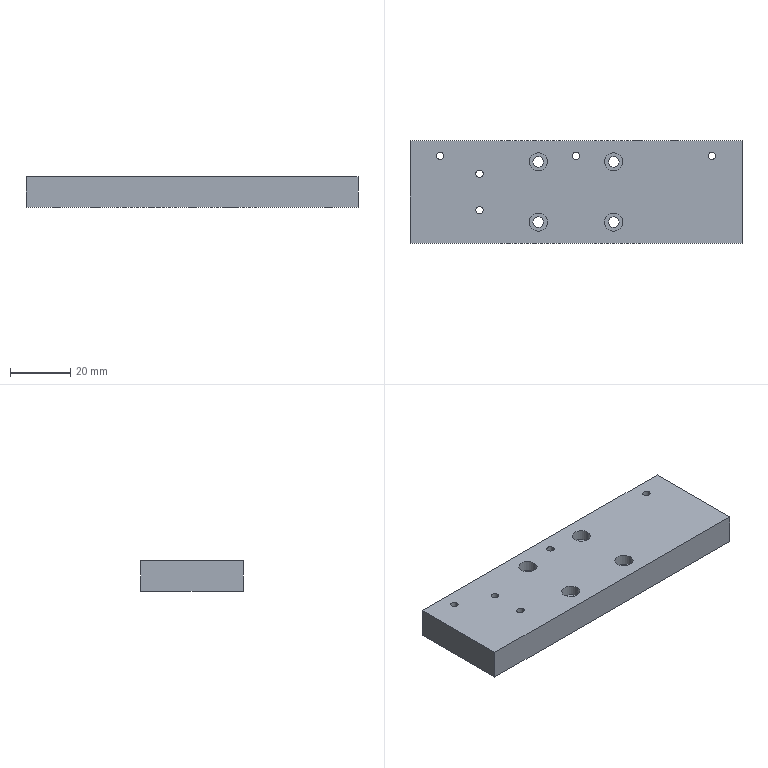Part | SolidWorks | features BaseBody 1 | 1 solid | 44 faces | box 110 x 34 x 10 mm | volume 36400 mm3 | cylinder 30 | plane 10 | cone 4 | commonest cylinder face diameters 2.459 x14 3.5 x8 6 x8
STEP:
#1=CARTESIAN_POINT('',(-17.191,-0.5864,0.));
#2=VERTEX_POINT('',#1);
#3=CARTESIAN_POINT('',(-20.691,-0.5864,0.));
#4=VERTEX_POINT('',#3);
#5=CARTESIAN_POINT('',(-18.941,-0.5864,0.));
#6=DIRECTION('',(0.,0.,-1.));
#7=DIRECTION('',(1.,0.,0.));
#8=AXIS2_PLACEMENT_3D('',#5,#6,#7);
#9=CIRCLE('',#8,1.75);
#10=EDGE_CURVE('',#2,#4,#9,.T.);
#11=ORIENTED_EDGE('',*,*,#10,.T.);
#12=CARTESIAN_POINT('',(-20.691,-0.5864,6.5));
#13=VERTEX_POINT('',#12);
#14=CARTESIAN_POINT('',(-20.691,-0.5864,-105.568));
#15=DIRECTION('',(0.,0.,1.));
#16=VECTOR('',#15,1000.);
#17=LINE('',#14,#16);
#18=EDGE_CURVE('',#4,#13,#17,.T.);
#19=ORIENTED_EDGE('',*,*,#18,.T.);
#20=CARTESIAN_POINT('',(-17.191,-0.5864,6.5));
#21=VERTEX_POINT('',#20);
#22=CARTESIAN_POINT('',(-18.941,-0.5864,6.5));
#23=DIRECTION('',(0.,0.,-1.));
#24=DIRECTION('',(1.,0.,0.));
#25=AXIS2_PLACEMENT_3D('',#22,#23,#24);
#26=CIRCLE('',#25,1.75);
#27=EDGE_CURVE('',#21,#13,#26,.T.);
#28=ORIENTED_EDGE('',*,*,#27,.F.);
#29=CARTESIAN_POINT('',(-17.191,-0.5864,-105.568));
#30=DIRECTION('',(0.,0.,1.));
#31=VECTOR('',#30,1000.);
#32=LINE('',#29,#31);
#33=EDGE_CURVE('',#2,#21,#32,.T.);
#34=ORIENTED_EDGE('',*,*,#33,.F.);
#35=EDGE_LOOP('',(#11,#19,#28,#34));
#36=FACE_OUTER_BOUND('',#35,.T.);
#37=CARTESIAN_POINT('',(-18.941,-0.5864,-105.568));
#38=DIRECTION('',(0.,0.,1.));
#39=DIRECTION('',(1.,0.,0.));
#40=AXIS2_PLACEMENT_3D('',#37,#38,#39);
#41=CYLINDRICAL_SURFACE('',#40,1.75);
#42=ADVANCED_FACE('',(#36),#41,.F.);
#43=CARTESIAN_POINT('',(7.809,-0.5864,0.));
#44=VERTEX_POINT('',#43);
#45=CARTESIAN_POINT('',(4.309,-0.5864,0.));
#46=VERTEX_POINT('',#45);
#47=CARTESIAN_POINT('',(6.059,-0.5864,0.));
#48=DIRECTION('',(0.,0.,-1.));
#49=DIRECTION('',(1.,0.,0.));
#50=AXIS2_PLACEMENT_3D('',#47,#48,#49);
#51=CIRCLE('',#50,1.75);
#52=EDGE_CURVE('',#44,#46,#51,.T.);
#53=ORIENTED_EDGE('',*,*,#52,.T.);
#54=CARTESIAN_POINT('',(4.309,-0.5864,6.5));
#55=VERTEX_POINT('',#54);
#56=CARTESIAN_POINT('',(4.309,-0.5864,-105.568));
#57=DIRECTION('',(0.,0.,1.));
#58=VECTOR('',#57,1000.);
#59=LINE('',#56,#58);
#60=EDGE_CURVE('',#46,#55,#59,.T.);
#61=ORIENTED_EDGE('',*,*,#60,.T.);
#62=CARTESIAN_POINT('',(7.809,-0.5864,6.5));
#63=VERTEX_POINT('',#62);
#64=CARTESIAN_POINT('',(6.059,-0.5864,6.5));
#65=DIRECTION('',(0.,0.,-1.));
#66=DIRECTION('',(1.,0.,0.));
#67=AXIS2_PLACEMENT_3D('',#64,#65,#66);
#68=CIRCLE('',#67,1.75);
#69=EDGE_CURVE('',#63,#55,#68,.T.);
#70=ORIENTED_EDGE('',*,*,#69,.F.);
#71=CARTESIAN_POINT('',(7.809,-0.5864,-105.568));
#72=DIRECTION('',(0.,0.,1.));
#73=VECTOR('',#72,1000.);
#74=LINE('',#71,#73);
#75=EDGE_CURVE('',#44,#63,#74,.T.);
#76=ORIENTED_EDGE('',*,*,#75,.F.);
#77=EDGE_LOOP('',(#53,#61,#70,#76));
#78=FACE_OUTER_BOUND('',#77,.T.);
#79=CARTESIAN_POINT('',(6.059,-0.5864,-105.568));
#80=DIRECTION('',(0.,0.,1.));
#81=DIRECTION('',(1.,0.,0.));
#82=AXIS2_PLACEMENT_3D('',#79,#80,#81);
#83=CYLINDRICAL_SURFACE('',#82,1.75);
#84=ADVANCED_FACE('',(#78),#83,.F.);
#85=CARTESIAN_POINT('',(7.809,-20.586,0.));
#86=VERTEX_POINT('',#85);
#87=CARTESIAN_POINT('',(4.309,-20.586,0.));
#88=VERTEX_POINT('',#87);
#89=CARTESIAN_POINT('',(6.059,-20.586,0.));
#90=DIRECTION('',(0.,0.,-1.));
#91=DIRECTION('',(1.,0.,0.));
#92=AXIS2_PLACEMENT_3D('',#89,#90,#91);
#93=CIRCLE('',#92,1.75);
#94=EDGE_CURVE('',#86,#88,#93,.T.);
#95=ORIENTED_EDGE('',*,*,#94,.T.);
#96=CARTESIAN_POINT('',(4.309,-20.586,6.5));
#97=VERTEX_POINT('',#96);
#98=CARTESIAN_POINT('',(4.309,-20.586,-105.568));
#99=DIRECTION('',(0.,0.,1.));
#100=VECTOR('',#99,1000.);
#101=LINE('',#98,#100);
#102=EDGE_CURVE('',#88,#97,#101,.T.);
#103=ORIENTED_EDGE('',*,*,#102,.T.);
#104=CARTESIAN_POINT('',(7.809,-20.586,6.5));
#105=VERTEX_POINT('',#104);
#106=CARTESIAN_POINT('',(6.059,-20.586,6.5));
#107=DIRECTION('',(0.,0.,-1.));
#108=DIRECTION('',(1.,0.,0.));
#109=AXIS2_PLACEMENT_3D('',#106,#107,#108);
#110=CIRCLE('',#109,1.75);
#111=EDGE_CURVE('',#105,#97,#110,.T.);
#112=ORIENTED_EDGE('',*,*,#111,.F.);
#113=CARTESIAN_POINT('',(7.809,-20.586,-105.568));
#114=DIRECTION('',(0.,0.,1.));
#115=VECTOR('',#114,1000.);
#116=LINE('',#113,#115);
#117=EDGE_CURVE('',#86,#105,#116,.T.);
#118=ORIENTED_EDGE('',*,*,#117,.F.);
#119=EDGE_LOOP('',(#95,#103,#112,#118));
#120=FACE_OUTER_BOUND('',#119,.T.);
#121=CARTESIAN_POINT('',(6.059,-20.586,-105.568));
#122=DIRECTION('',(0.,0.,1.));
#123=DIRECTION('',(1.,0.,0.));
#124=AXIS2_PLACEMENT_3D('',#121,#122,#123);
#125=CYLINDRICAL_SURFACE('',#124,1.75);
#126=ADVANCED_FACE('',(#120),#125,.F.);
#127=CARTESIAN_POINT('',(-17.191,-20.586,0.));
#128=VERTEX_POINT('',#127);
#129=CARTESIAN_POINT('',(-20.691,-20.586,0.));
#130=VERTEX_POINT('',#129);
#131=CARTESIAN_POINT('',(-18.941,-20.586,0.));
#132=DIRECTION('',(0.,0.,-1.));
#133=DIRECTION('',(1.,0.,0.));
#134=AXIS2_PLACEMENT_3D('',#131,#132,#133);
#135=CIRCLE('',#134,1.75);
#136=EDGE_CURVE('',#128,#130,#135,.T.);
#137=ORIENTED_EDGE('',*,*,#136,.T.);
#138=CARTESIAN_POINT('',(-20.691,-20.586,6.5));
#139=VERTEX_POINT('',#138);
#140=CARTESIAN_POINT('',(-20.691,-20.586,-105.568));
#141=DIRECTION('',(0.,0.,1.));
#142=VECTOR('',#141,1000.);
#143=LINE('',#140,#142);
#144=EDGE_CURVE('',#130,#139,#143,.T.);
#145=ORIENTED_EDGE('',*,*,#144,.T.);
#146=CARTESIAN_POINT('',(-17.191,-20.586,6.5));
#147=VERTEX_POINT('',#146);
#148=CARTESIAN_POINT('',(-18.941,-20.586,6.5));
#149=DIRECTION('',(0.,0.,-1.));
#150=DIRECTION('',(1.,0.,0.));
#151=AXIS2_PLACEMENT_3D('',#148,#149,#150);
#152=CIRCLE('',#151,1.75);
#153=EDGE_CURVE('',#147,#139,#152,.T.);
#154=ORIENTED_EDGE('',*,*,#153,.F.);
#155=CARTESIAN_POINT('',(-17.191,-20.586,-105.568));
#156=DIRECTION('',(0.,0.,1.));
#157=VECTOR('',#156,1000.);
#158=LINE('',#155,#157);
#159=EDGE_CURVE('',#128,#147,#158,.T.);
#160=ORIENTED_EDGE('',*,*,#159,.F.);
#161=EDGE_LOOP('',(#137,#145,#154,#160));
#162=FACE_OUTER_BOUND('',#161,.T.);
#163=CARTESIAN_POINT('',(-18.941,-20.586,-105.568));
#164=DIRECTION('',(0.,0.,1.));
#165=DIRECTION('',(1.,0.,0.));
#166=AXIS2_PLACEMENT_3D('',#163,#164,#165);
#167=CYLINDRICAL_SURFACE('',#166,1.75);
#168=ADVANCED_FACE('',(#162),#167,.F.);
#169=CARTESIAN_POINT('',(-50.211,1.414,0.));
#170=VERTEX_POINT('',#169);
#171=CARTESIAN_POINT('',(-52.67,1.414,0.));
#172=VERTEX_POINT('',#171);
#173=CARTESIAN_POINT('',(-51.441,1.414,0.));
#174=DIRECTION('',(0.,0.,-1.));
#175=DIRECTION('',(1.,0.,0.));
#176=AXIS2_PLACEMENT_3D('',#173,#174,#175);
#177=CIRCLE('',#176,1.23);
#178=EDGE_CURVE('',#170,#172,#177,.T.);
#179=ORIENTED_EDGE('',*,*,#178,.T.);
#180=CARTESIAN_POINT('',(-52.67,1.414,10.));
#181=VERTEX_POINT('',#180);
#182=CARTESIAN_POINT('',(-52.67,1.414,-105.568));
#183=DIRECTION('',(0.,0.,1.));
#184=VECTOR('',#183,1000.);
#185=LINE('',#182,#184);
#186=EDGE_CURVE('',#172,#181,#185,.T.);
#187=ORIENTED_EDGE('',*,*,#186,.T.);
#188=CARTESIAN_POINT('',(-50.211,1.414,10.));
#189=VERTEX_POINT('',#188);
#190=CARTESIAN_POINT('',(-51.441,1.414,10.));
#191=DIRECTION('',(0.,0.,-1.));
#192=DIRECTION('',(1.,0.,0.));
#193=AXIS2_PLACEMENT_3D('',#190,#191,#192);
#194=CIRCLE('',#193,1.23);
#195=EDGE_CURVE('',#189,#181,#194,.T.);
#196=ORIENTED_EDGE('',*,*,#195,.F.);
#197=CARTESIAN_POINT('',(-50.211,1.414,-105.568));
#198=DIRECTION('',(0.,0.,1.));
#199=VECTOR('',#198,1000.);
#200=LINE('',#197,#199);
#201=EDGE_CURVE('',#170,#189,#200,.T.);
#202=ORIENTED_EDGE('',*,*,#201,.F.);
#203=EDGE_LOOP('',(#179,#187,#196,#202));
#204=FACE_OUTER_BOUND('',#203,.T.);
#205=CARTESIAN_POINT('',(-51.441,1.414,-105.568));
#206=DIRECTION('',(0.,0.,1.));
#207=DIRECTION('',(1.,0.,0.));
#208=AXIS2_PLACEMENT_3D('',#205,#206,#207);
#209=CYLINDRICAL_SURFACE('',#208,1.23);
#210=ADVANCED_FACE('',(#204),#209,.F.);
#211=CARTESIAN_POINT('',(-5.211,1.414,0.));
#212=VERTEX_POINT('',#211);
#213=CARTESIAN_POINT('',(-7.67,1.414,0.));
#214=VERTEX_POINT('',#213);
#215=CARTESIAN_POINT('',(-6.441,1.414,0.));
#216=DIRECTION('',(0.,0.,-1.));
#217=DIRECTION('',(1.,0.,0.));
#218=AXIS2_PLACEMENT_3D('',#215,#216,#217);
#219=CIRCLE('',#218,1.229);
#220=EDGE_CURVE('',#212,#214,#219,.T.);
#221=ORIENTED_EDGE('',*,*,#220,.T.);
#222=CARTESIAN_POINT('',(-7.67,1.414,10.));
#223=VERTEX_POINT('',#222);
#224=CARTESIAN_POINT('',(-7.67,1.414,-105.568));
#225=DIRECTION('',(0.,0.,1.));
#226=VECTOR('',#225,1000.);
#227=LINE('',#224,#226);
#228=EDGE_CURVE('',#214,#223,#227,.T.);
#229=ORIENTED_EDGE('',*,*,#228,.T.);
#230=CARTESIAN_POINT('',(-5.211,1.414,10.));
#231=VERTEX_POINT('',#230);
#232=CARTESIAN_POINT('',(-6.441,1.414,10.));
#233=DIRECTION('',(0.,0.,-1.));
#234=DIRECTION('',(1.,0.,0.));
#235=AXIS2_PLACEMENT_3D('',#232,#233,#234);
#236=CIRCLE('',#235,1.229);
#237=EDGE_CURVE('',#231,#223,#236,.T.);
#238=ORIENTED_EDGE('',*,*,#237,.F.);
#239=CARTESIAN_POINT('',(-5.211,1.414,-105.568));
#240=DIRECTION('',(0.,0.,1.));
#241=VECTOR('',#240,1000.);
#242=LINE('',#239,#241);
#243=EDGE_CURVE('',#212,#231,#242,.T.);
#244=ORIENTED_EDGE('',*,*,#243,.F.);
#245=EDGE_LOOP('',(#221,#229,#238,#244));
#246=FACE_OUTER_BOUND('',#245,.T.);
#247=CARTESIAN_POINT('',(-6.441,1.414,-105.568));
#248=DIRECTION('',(0.,0.,1.));
#249=DIRECTION('',(1.,0.,0.));
#250=AXIS2_PLACEMENT_3D('',#247,#248,#249);
#251=CYLINDRICAL_SURFACE('',#250,1.229);
#252=ADVANCED_FACE('',(#246),#251,.F.);
#253=CARTESIAN_POINT('',(39.789,1.414,0.));
#254=VERTEX_POINT('',#253);
#255=CARTESIAN_POINT('',(37.33,1.414,0.));
#256=VERTEX_POINT('',#255);
#257=CARTESIAN_POINT('',(38.559,1.414,0.));
#258=DIRECTION('',(0.,0.,-1.));
#259=DIRECTION('',(1.,0.,0.));
#260=AXIS2_PLACEMENT_3D('',#257,#258,#259);
#261=CIRCLE('',#260,1.23);
#262=EDGE_CURVE('',#254,#256,#261,.T.);
#263=ORIENTED_EDGE('',*,*,#262,.T.);
#264=CARTESIAN_POINT('',(37.33,1.414,10.));
#265=VERTEX_POINT('',#264);
#266=CARTESIAN_POINT('',(37.33,1.414,-105.568));
#267=DIRECTION('',(0.,0.,1.));
#268=VECTOR('',#267,1000.);
#269=LINE('',#266,#268);
#270=EDGE_CURVE('',#256,#265,#269,.T.);
#271=ORIENTED_EDGE('',*,*,#270,.T.);
#272=CARTESIAN_POINT('',(39.789,1.414,10.));
#273=VERTEX_POINT('',#272);
#274=CARTESIAN_POINT('',(38.559,1.414,10.));
#275=DIRECTION('',(0.,0.,-1.));
#276=DIRECTION('',(1.,0.,0.));
#277=AXIS2_PLACEMENT_3D('',#274,#275,#276);
#278=CIRCLE('',#277,1.23);
#279=EDGE_CURVE('',#273,#265,#278,.T.);
#280=ORIENTED_EDGE('',*,*,#279,.F.);
#281=CARTESIAN_POINT('',(39.789,1.414,-105.568));
#282=DIRECTION('',(0.,0.,1.));
#283=VECTOR('',#282,1000.);
#284=LINE('',#281,#283);
#285=EDGE_CURVE('',#254,#273,#284,.T.);
#286=ORIENTED_EDGE('',*,*,#285,.F.);
#287=EDGE_LOOP('',(#263,#271,#280,#286));
#288=FACE_OUTER_BOUND('',#287,.T.);
#289=CARTESIAN_POINT('',(38.559,1.414,-105.568));
#290=DIRECTION('',(0.,0.,1.));
#291=DIRECTION('',(1.,0.,0.));
#292=AXIS2_PLACEMENT_3D('',#289,#290,#291);
#293=CYLINDRICAL_SURFACE('',#292,1.23);
#294=ADVANCED_FACE('',(#288),#293,.F.);
#295=CARTESIAN_POINT('',(-37.211,-4.586,10.));
#296=VERTEX_POINT('',#295);
#297=CARTESIAN_POINT('',(-39.67,-4.586,10.));
#298=VERTEX_POINT('',#297);
#299=CARTESIAN_POINT('',(-38.441,-4.586,10.));
#300=DIRECTION('',(0.,0.,-1.));
#301=DIRECTION('',(-1.,0.,0.));
#302=AXIS2_PLACEMENT_3D('',#299,#300,#301);
#303=CIRCLE('',#302,1.23);
#304=EDGE_CURVE('',#296,#298,#303,.T.);
#305=ORIENTED_EDGE('',*,*,#304,.F.);
#306=CARTESIAN_POINT('',(-37.211,-4.586,0.));
#307=VERTEX_POINT('',#306);
#308=CARTESIAN_POINT('',(-37.211,-4.586,115.568));
#309=DIRECTION('',(0.,0.,-1.));
#310=VECTOR('',#309,1000.);
#311=LINE('',#308,#310);
#312=EDGE_CURVE('',#296,#307,#311,.T.);
#313=ORIENTED_EDGE('',*,*,#312,.T.);
#314=CARTESIAN_POINT('',(-39.67,-4.586,0.));
#315=VERTEX_POINT('',#314);
#316=CARTESIAN_POINT('',(-38.441,-4.586,0.));
#317=DIRECTION('',(0.,0.,-1.));
#318=DIRECTION('',(-1.,0.,0.));
#319=AXIS2_PLACEMENT_3D('',#316,#317,#318);
#320=CIRCLE('',#319,1.23);
#321=EDGE_CURVE('',#307,#315,#320,.T.);
#322=ORIENTED_EDGE('',*,*,#321,.T.);
#323=CARTESIAN_POINT('',(-39.67,-4.586,115.568));
#324=DIRECTION('',(0.,0.,-1.));
#325=VECTOR('',#324,1000.);
#326=LINE('',#323,#325);
#327=EDGE_CURVE('',#298,#315,#326,.T.);
#328=ORIENTED_EDGE('',*,*,#327,.F.);
#329=EDGE_LOOP('',(#305,#313,#322,#328));
#330=FACE_OUTER_BOUND('',#329,.T.);
#331=CARTESIAN_POINT('',(-38.441,-4.586,115.568));
#332=DIRECTION('',(0.,0.,-1.));
#333=DIRECTION('',(-1.,0.,0.));
#334=AXIS2_PLACEMENT_3D('',#331,#332,#333);
#335=CYLINDRICAL_SURFACE('',#334,1.23);
#336=ADVANCED_FACE('',(#330),#335,.F.);
#337=CARTESIAN_POINT('',(-37.211,-16.586,10.));
#338=VERTEX_POINT('',#337);
#339=CARTESIAN_POINT('',(-39.67,-16.586,10.));
#340=VERTEX_POINT('',#339);
#341=CARTESIAN_POINT('',(-38.441,-16.586,10.));
#342=DIRECTION('',(0.,0.,-1.));
#343=DIRECTION('',(-1.,0.,0.));
#344=AXIS2_PLACEMENT_3D('',#341,#342,#343);
#345=CIRCLE('',#344,1.23);
#346=EDGE_CURVE('',#338,#340,#345,.T.);
#347=ORIENTED_EDGE('',*,*,#346,.F.);
#348=CARTESIAN_POINT('',(-37.211,-16.586,0.));
#349=VERTEX_POINT('',#348);
#350=CARTESIAN_POINT('',(-37.211,-16.586,115.568));
#351=DIRECTION('',(0.,0.,-1.));
#352=VECTOR('',#351,1000.);
#353=LINE('',#350,#352);
#354=EDGE_CURVE('',#338,#349,#353,.T.);
#355=ORIENTED_EDGE('',*,*,#354,.T.);
#356=CARTESIAN_POINT('',(-39.67,-16.586,0.));
#357=VERTEX_POINT('',#356);
#358=CARTESIAN_POINT('',(-38.441,-16.586,0.));
#359=DIRECTION('',(0.,0.,-1.));
#360=DIRECTION('',(-1.,0.,0.));
#361=AXIS2_PLACEMENT_3D('',#358,#359,#360);
#362=CIRCLE('',#361,1.23);
#363=EDGE_CURVE('',#349,#357,#362,.T.);
#364=ORIENTED_EDGE('',*,*,#363,.T.);
#365=CARTESIAN_POINT('',(-39.67,-16.586,115.568));
#366=DIRECTION('',(0.,0.,-1.));
#367=VECTOR('',#366,1000.);
#368=LINE('',#365,#367);
#369=EDGE_CURVE('',#340,#357,#368,.T.);
#370=ORIENTED_EDGE('',*,*,#369,.F.);
#371=EDGE_LOOP('',(#347,#355,#364,#370));
#372=FACE_OUTER_BOUND('',#371,.T.);
#373=CARTESIAN_POINT('',(-38.441,-16.586,115.568));
#374=DIRECTION('',(0.,0.,-1.));
#375=DIRECTION('',(-1.,0.,0.));
#376=AXIS2_PLACEMENT_3D('',#373,#374,#375);
#377=CYLINDRICAL_SURFACE('',#376,1.23);
#378=ADVANCED_FACE('',(#372),#377,.F.);
#379=CARTESIAN_POINT('',(14.059,-5.586,1.771));
#380=VERTEX_POINT('',#379);
#381=CARTESIAN_POINT('',(14.059,-5.586,4.229));
#382=VERTEX_POINT('',#381);
#383=CARTESIAN_POINT('',(14.059,-5.586,3.));
#384=DIRECTION('',(0.,1.,0.));
#385=DIRECTION('',(0.,0.,1.));
#386=AXIS2_PLACEMENT_3D('',#383,#384,#385);
#387=CIRCLE('',#386,1.229);
#388=EDGE_CURVE('',#380,#382,#387,.T.);
#389=ORIENTED_EDGE('',*,*,#388,.F.);
#390=CARTESIAN_POINT('',(14.059,6.414,1.771));
#391=VERTEX_POINT('',#390);
#392=CARTESIAN_POINT('',(14.059,0.4136,1.771));
#393=DIRECTION('',(0.,1.,0.));
#394=VECTOR('',#393,1000.);
#395=LINE('',#392,#394);
#396=EDGE_CURVE('',#380,#391,#395,.T.);
#397=ORIENTED_EDGE('',*,*,#396,.T.);
#398=CARTESIAN_POINT('',(14.059,6.414,4.23));
#399=VERTEX_POINT('',#398);
#400=CARTESIAN_POINT('',(14.059,6.414,3.));
#401=DIRECTION('',(0.,-1.,0.));
#402=DIRECTION('',(0.,0.,1.));
#403=AXIS2_PLACEMENT_3D('',#400,#401,#402);
#404=CIRCLE('',#403,1.229);
#405=EDGE_CURVE('',#399,#391,#404,.T.);
#406=ORIENTED_EDGE('',*,*,#405,.F.);
#407=CARTESIAN_POINT('',(14.059,0.4136,4.23));
#408=DIRECTION('',(0.,1.,0.));
#409=VECTOR('',#408,1000.);
#410=LINE('',#407,#409);
#411=EDGE_CURVE('',#382,#399,#410,.T.);
#412=ORIENTED_EDGE('',*,*,#411,.F.);
#413=EDGE_LOOP('',(#389,#397,#406,#412));
#414=FACE_OUTER_BOUND('',#413,.T.);
#415=CARTESIAN_POINT('',(14.059,0.4136,3.));
#416=DIRECTION('',(0.,1.,0.));
#417=DIRECTION('',(0.,0.,1.));
#418=AXIS2_PLACEMENT_3D('',#415,#416,#417);
#419=CYLINDRICAL_SURFACE('',#418,1.229);
#420=ADVANCED_FACE('',(#414),#419,.F.);
#421=CARTESIAN_POINT('',(26.059,-5.586,1.771));
#422=VERTEX_POINT('',#421);
#423=CARTESIAN_POINT('',(26.059,-5.586,4.229));
#424=VERTEX_POINT('',#423);
#425=CARTESIAN_POINT('',(26.059,-5.586,3.));
#426=DIRECTION('',(0.,1.,0.));
#427=DIRECTION('',(0.,0.,1.));
#428=AXIS2_PLACEMENT_3D('',#425,#426,#427);
#429=CIRCLE('',#428,1.23);
#430=EDGE_CURVE('',#422,#424,#429,.T.);
#431=ORIENTED_EDGE('',*,*,#430,.F.);
#432=CARTESIAN_POINT('',(26.059,6.414,1.771));
#433=VERTEX_POINT('',#432);
#434=CARTESIAN_POINT('',(26.059,0.4136,1.771));
#435=DIRECTION('',(0.,1.,0.));
#436=VECTOR('',#435,1000.);
#437=LINE('',#434,#436);
#438=EDGE_CURVE('',#422,#433,#437,.T.);
#439=ORIENTED_EDGE('',*,*,#438,.T.);
#440=CARTESIAN_POINT('',(26.059,6.414,4.23));
#441=VERTEX_POINT('',#440);
#442=CARTESIAN_POINT('',(26.059,6.414,3.));
#443=DIRECTION('',(0.,-1.,0.));
#444=DIRECTION('',(0.,0.,1.));
#445=AXIS2_PLACEMENT_3D('',#442,#443,#444);
#446=CIRCLE('',#445,1.23);
#447=EDGE_CURVE('',#441,#433,#446,.T.);
#448=ORIENTED_EDGE('',*,*,#447,.F.);
#449=CARTESIAN_POINT('',(26.059,0.4136,4.23));
#450=DIRECTION('',(0.,1.,0.));
#451=VECTOR('',#450,1000.);
#452=LINE('',#449,#451);
#453=EDGE_CURVE('',#424,#441,#452,.T.);
#454=ORIENTED_EDGE('',*,*,#453,.F.);
#455=EDGE_LOOP('',(#431,#439,#448,#454));
#456=FACE_OUTER_BOUND('',#455,.T.);
#457=CARTESIAN_POINT('',(26.059,0.4136,3.));
#458=DIRECTION('',(0.,1.,0.));
#459=DIRECTION('',(0.,0.,1.));
#460=AXIS2_PLACEMENT_3D('',#457,#458,#459);
#461=CYLINDRICAL_SURFACE('',#460,1.23);
#462=ADVANCED_FACE('',(#456),#461,.F.);
#463=CARTESIAN_POINT('',(-21.941,-0.5864,6.5));
#464=VERTEX_POINT('',#463);
#465=CARTESIAN_POINT('',(-15.941,-0.5864,6.5));
#466=VERTEX_POINT('',#465);
#467=CARTESIAN_POINT('',(-18.941,-0.5864,6.5));
#468=DIRECTION('',(0.,0.,1.));
#469=DIRECTION('',(1.,0.,0.));
#470=AXIS2_PLACEMENT_3D('',#467,#468,#469);
#471=CIRCLE('',#470,3.);
#472=EDGE_CURVE('',#464,#466,#471,.T.);
#473=ORIENTED_EDGE('',*,*,#472,.F.);
#474=CARTESIAN_POINT('',(-21.941,-0.5864,10.));
#475=VERTEX_POINT('',#474);
#476=CARTESIAN_POINT('',(-21.941,-0.5864,8.25));
#477=DIRECTION('',(0.,0.,1.));
#478=VECTOR('',#477,1000.);
#479=LINE('',#476,#478);
#480=EDGE_CURVE('',#464,#475,#479,.T.);
#481=ORIENTED_EDGE('',*,*,#480,.T.);
#482=CARTESIAN_POINT('',(-15.941,-0.5864,10.));
#483=VERTEX_POINT('',#482);
#484=CARTESIAN_POINT('',(-18.941,-0.5864,10.));
#485=DIRECTION('',(0.,0.,-1.));
#486=DIRECTION('',(1.,0.,0.));
#487=AXIS2_PLACEMENT_3D('',#484,#485,#486);
#488=CIRCLE('',#487,3.);
#489=EDGE_CURVE('',#483,#475,#488,.T.);
#490=ORIENTED_EDGE('',*,*,#489,.F.);
#491=CARTESIAN_POINT('',(-15.941,-0.5864,8.25));
#492=DIRECTION('',(0.,0.,1.));
#493=VECTOR('',#492,1000.);
#494=LINE('',#491,#493);
#495=EDGE_CURVE('',#466,#483,#494,.T.);
#496=ORIENTED_EDGE('',*,*,#495,.F.);
#497=EDGE_LOOP('',(#473,#481,#490,#496));
#498=FACE_OUTER_BOUND('',#497,.T.);
#499=CARTESIAN_POINT('',(-18.941,-0.5864,8.25));
#500=DIRECTION('',(0.,0.,1.));
#501=DIRECTION('',(1.,0.,0.));
#502=AXIS2_PLACEMENT_3D('',#499,#500,#501);
#503=CYLINDRICAL_SURFACE('',#502,3.);
#504=ADVANCED_FACE('',(#498),#503,.F.);
#505=CARTESIAN_POINT('',(3.059,-0.5864,6.5));
#506=VERTEX_POINT('',#505);
#507=CARTESIAN_POINT('',(9.059,-0.5864,6.5));
#508=VERTEX_POINT('',#507);
#509=CARTESIAN_POINT('',(6.059,-0.5864,6.5));
#510=DIRECTION('',(0.,0.,1.));
#511=DIRECTION('',(1.,0.,0.));
#512=AXIS2_PLACEMENT_3D('',#509,#510,#511);
#513=CIRCLE('',#512,3.);
#514=EDGE_CURVE('',#506,#508,#513,.T.);
#515=ORIENTED_EDGE('',*,*,#514,.F.);
#516=CARTESIAN_POINT('',(3.059,-0.5864,10.));
#517=VERTEX_POINT('',#516);
#518=CARTESIAN_POINT('',(3.059,-0.5864,8.25));
#519=DIRECTION('',(0.,0.,1.));
#520=VECTOR('',#519,1000.);
#521=LINE('',#518,#520);
#522=EDGE_CURVE('',#506,#517,#521,.T.);
#523=ORIENTED_EDGE('',*,*,#522,.T.);
#524=CARTESIAN_POINT('',(9.059,-0.5864,10.));
#525=VERTEX_POINT('',#524);
#526=CARTESIAN_POINT('',(6.059,-0.5864,10.));
#527=DIRECTION('',(0.,0.,-1.));
#528=DIRECTION('',(1.,0.,0.));
#529=AXIS2_PLACEMENT_3D('',#526,#527,#528);
#530=CIRCLE('',#529,3.);
#531=EDGE_CURVE('',#525,#517,#530,.T.);
#532=ORIENTED_EDGE('',*,*,#531,.F.);
#533=CARTESIAN_POINT('',(9.059,-0.5864,8.25));
#534=DIRECTION('',(0.,0.,1.));
#535=VECTOR('',#534,1000.);
#536=LINE('',#533,#535);
#537=EDGE_CURVE('',#508,#525,#536,.T.);
#538=ORIENTED_EDGE('',*,*,#537,.F.);
#539=EDGE_LOOP('',(#515,#523,#532,#538));
#540=FACE_OUTER_BOUND('',#539,.T.);
#541=CARTESIAN_POINT('',(6.059,-0.5864,8.25));
#542=DIRECTION('',(0.,0.,1.));
#543=DIRECTION('',(1.,0.,0.));
#544=AXIS2_PLACEMENT_3D('',#541,#542,#543);
#545=CYLINDRICAL_SURFACE('',#544,3.);
#546=ADVANCED_FACE('',(#540),#545,.F.);
#547=CARTESIAN_POINT('',(3.059,-20.586,6.5));
#548=VERTEX_POINT('',#547);
#549=CARTESIAN_POINT('',(9.059,-20.586,6.5));
#550=VERTEX_POINT('',#549);
#551=CARTESIAN_POINT('',(6.059,-20.586,6.5));
#552=DIRECTION('',(0.,0.,1.));
#553=DIRECTION('',(1.,0.,0.));
#554=AXIS2_PLACEMENT_3D('',#551,#552,#553);
#555=CIRCLE('',#554,3.);
#556=EDGE_CURVE('',#548,#550,#555,.T.);
#557=ORIENTED_EDGE('',*,*,#556,.F.);
#558=CARTESIAN_POINT('',(3.059,-20.586,10.));
#559=VERTEX_POINT('',#558);
#560=CARTESIAN_POINT('',(3.059,-20.586,8.25));
#561=DIRECTION('',(0.,0.,1.));
#562=VECTOR('',#561,1000.);
#563=LINE('',#560,#562);
#564=EDGE_CURVE('',#548,#559,#563,.T.);
#565=ORIENTED_EDGE('',*,*,#564,.T.);
#566=CARTESIAN_POINT('',(9.059,-20.586,10.));
#567=VERTEX_POINT('',#566);
#568=CARTESIAN_POINT('',(6.059,-20.586,10.));
#569=DIRECTION('',(0.,0.,-1.));
#570=DIRECTION('',(1.,0.,0.));
#571=AXIS2_PLACEMENT_3D('',#568,#569,#570);
#572=CIRCLE('',#571,3.);
#573=EDGE_CURVE('',#567,#559,#572,.T.);
#574=ORIENTED_EDGE('',*,*,#573,.F.);
#575=CARTESIAN_POINT('',(9.059,-20.586,8.25));
#576=DIRECTION('',(0.,0.,1.));
#577=VECTOR('',#576,1000.);
#578=LINE('',#575,#577);
#579=EDGE_CURVE('',#550,#567,#578,.T.);
#580=ORIENTED_EDGE('',*,*,#579,.F.);
#581=EDGE_LOOP('',(#557,#565,#574,#580));
#582=FACE_OUTER_BOUND('',#581,.T.);
#583=CARTESIAN_POINT('',(6.059,-20.586,8.25));
#584=DIRECTION('',(0.,0.,1.));
#585=DIRECTION('',(1.,0.,0.));
#586=AXIS2_PLACEMENT_3D('',#583,#584,#585);
#587=CYLINDRICAL_SURFACE('',#586,3.);
#588=ADVANCED_FACE('',(#582),#587,.F.);
#589=CARTESIAN_POINT('',(-21.941,-20.586,6.5));
#590=VERTEX_POINT('',#589);
#591=CARTESIAN_POINT('',(-15.941,-20.586,6.5));
#592=VERTEX_POINT('',#591);
#593=CARTESIAN_POINT('',(-18.941,-20.586,6.5));
#594=DIRECTION('',(0.,0.,1.));
#595=DIRECTION('',(1.,0.,0.));
#596=AXIS2_PLACEMENT_3D('',#593,#594,#595);
#597=CIRCLE('',#596,3.);
#598=EDGE_CURVE('',#590,#592,#597,.T.);
#599=ORIENTED_EDGE('',*,*,#598,.F.);
#600=CARTESIAN_POINT('',(-21.941,-20.586,10.));
#601=VERTEX_POINT('',#600);
#602=CARTESIAN_POINT('',(-21.941,-20.586,8.25));
#603=DIRECTION('',(0.,0.,1.));
#604=VECTOR('',#603,1000.);
#605=LINE('',#602,#604);
#606=EDGE_CURVE('',#590,#601,#605,.T.);
#607=ORIENTED_EDGE('',*,*,#606,.T.);
#608=CARTESIAN_POINT('',(-15.941,-20.586,10.));
#609=VERTEX_POINT('',#608);
#610=CARTESIAN_POINT('',(-18.941,-20.586,10.));
#611=DIRECTION('',(0.,0.,-1.));
#612=DIRECTION('',(1.,0.,0.));
#613=AXIS2_PLACEMENT_3D('',#610,#611,#612);
#614=CIRCLE('',#613,3.);
#615=EDGE_CURVE('',#609,#601,#614,.T.);
#616=ORIENTED_EDGE('',*,*,#615,.F.);
#617=CARTESIAN_POINT('',(-15.941,-20.586,8.25));
#618=DIRECTION('',(0.,0.,1.));
#619=VECTOR('',#618,1000.);
#620=LINE('',#617,#619);
#621=EDGE_CURVE('',#592,#609,#620,.T.);
#622=ORIENTED_EDGE('',*,*,#621,.F.);
#623=EDGE_LOOP('',(#599,#607,#616,#622));
#624=FACE_OUTER_BOUND('',#623,.T.);
#625=CARTESIAN_POINT('',(-18.941,-20.586,8.25));
#626=DIRECTION('',(0.,0.,1.));
#627=DIRECTION('',(1.,0.,0.));
#628=AXIS2_PLACEMENT_3D('',#625,#626,#627);
#629=CYLINDRICAL_SURFACE('',#628,3.);
#630=ADVANCED_FACE('',(#624),#629,.F.);
#631=CARTESIAN_POINT('',(14.059,-6.325,3.));
#632=VERTEX_POINT('',#631);
#633=CARTESIAN_POINT('',(14.059,-5.586,4.229));
#634=DIRECTION('',(0.,0.515,0.8572));
#635=VECTOR('',#634,1000.);
#636=LINE('',#633,#635);
#637=EDGE_CURVE('',#632,#382,#636,.T.);
#638=ORIENTED_EDGE('',*,*,#637,.F.);
#639=CARTESIAN_POINT('',(14.059,-5.586,1.771));
#640=DIRECTION('',(0.,0.515,-0.8572));
#641=VECTOR('',#640,1000.);
#642=LINE('',#639,#641);
#643=EDGE_CURVE('',#632,#380,#642,.T.);
#644=ORIENTED_EDGE('',*,*,#643,.T.);
#645=ORIENTED_EDGE('',*,*,#388,.T.);
#646=EDGE_LOOP('',(#638,#644,#645));
#647=FACE_OUTER_BOUND('',#646,.T.);
#648=CARTESIAN_POINT('',(14.059,-5.586,3.));
#649=DIRECTION('',(0.,1.,0.));
#650=DIRECTION('',(0.,0.,1.));
#651=AXIS2_PLACEMENT_3D('',#648,#649,#650);
#652=CONICAL_SURFACE('',#651,1.229,1.03);
#653=ADVANCED_FACE('',(#647),#652,.F.);
#654=CARTESIAN_POINT('',(26.059,-6.325,3.));
#655=VERTEX_POINT('',#654);
#656=CARTESIAN_POINT('',(26.059,-5.586,4.229));
#657=DIRECTION('',(0.,0.515,0.8572));
#658=VECTOR('',#657,1000.);
#659=LINE('',#656,#658);
#660=EDGE_CURVE('',#655,#424,#659,.T.);
#661=ORIENTED_EDGE('',*,*,#660,.F.);
#662=CARTESIAN_POINT('',(26.059,-5.586,1.771));
#663=DIRECTION('',(0.,0.515,-0.8572));
#664=VECTOR('',#663,1000.);
#665=LINE('',#662,#664);
#666=EDGE_CURVE('',#655,#422,#665,.T.);
#667=ORIENTED_EDGE('',*,*,#666,.T.);
#668=ORIENTED_EDGE('',*,*,#430,.T.);
#669=EDGE_LOOP('',(#661,#667,#668));
#670=FACE_OUTER_BOUND('',#669,.T.);
#671=CARTESIAN_POINT('',(26.059,-5.586,3.));
#672=DIRECTION('',(0.,1.,0.));
#673=DIRECTION('',(0.,0.,1.));
#674=AXIS2_PLACEMENT_3D('',#671,#672,#673);
#675=CONICAL_SURFACE('',#674,1.229,1.03);
#676=ADVANCED_FACE('',(#670),#675,.F.);
#677=ORIENTED_EDGE('',*,*,#10,.F.);
#678=CARTESIAN_POINT('',(-18.941,-0.5864,0.));
#679=DIRECTION('',(0.,0.,-1.));
#680=DIRECTION('',(1.,0.,0.));
#681=AXIS2_PLACEMENT_3D('',#678,#679,#680);
#682=CIRCLE('',#681,1.75);
#683=EDGE_CURVE('',#4,#2,#682,.T.);
#684=ORIENTED_EDGE('',*,*,#683,.F.);
#685=EDGE_LOOP('',(#677,#684));
#686=FACE_BOUND('',#685,.T.);
#687=ORIENTED_EDGE('',*,*,#52,.F.);
#688=CARTESIAN_POINT('',(6.059,-0.5864,0.));
#689=DIRECTION('',(0.,0.,-1.));
#690=DIRECTION('',(1.,0.,0.));
#691=AXIS2_PLACEMENT_3D('',#688,#689,#690);
#692=CIRCLE('',#691,1.75);
#693=EDGE_CURVE('',#46,#44,#692,.T.);
#694=ORIENTED_EDGE('',*,*,#693,.F.);
#695=EDGE_LOOP('',(#687,#694));
#696=FACE_BOUND('',#695,.T.);
#697=ORIENTED_EDGE('',*,*,#94,.F.);
#698=CARTESIAN_POINT('',(6.059,-20.586,0.));
#699=DIRECTION('',(0.,0.,-1.));
#700=DIRECTION('',(1.,0.,0.));
#701=AXIS2_PLACEMENT_3D('',#698,#699,#700);
#702=CIRCLE('',#701,1.75);
#703=EDGE_CURVE('',#88,#86,#702,.T.);
#704=ORIENTED_EDGE('',*,*,#703,.F.);
#705=EDGE_LOOP('',(#697,#704));
#706=FACE_BOUND('',#705,.T.);
#707=ORIENTED_EDGE('',*,*,#136,.F.);
#708=CARTESIAN_POINT('',(-18.941,-20.586,0.));
#709=DIRECTION('',(0.,0.,-1.));
#710=DIRECTION('',(1.,0.,0.));
#711=AXIS2_PLACEMENT_3D('',#708,#709,#710);
#712=CIRCLE('',#711,1.75);
#713=EDGE_CURVE('',#130,#128,#712,.T.);
#714=ORIENTED_EDGE('',*,*,#713,.F.);
#715=EDGE_LOOP('',(#707,#714));
#716=FACE_BOUND('',#715,.T.);
#717=ORIENTED_EDGE('',*,*,#178,.F.);
#718=CARTESIAN_POINT('',(-51.441,1.414,0.));
#719=DIRECTION('',(0.,0.,-1.));
#720=DIRECTION('',(1.,0.,0.));
#721=AXIS2_PLACEMENT_3D('',#718,#719,#720);
#722=CIRCLE('',#721,1.23);
#723=EDGE_CURVE('',#172,#170,#722,.T.);
#724=ORIENTED_EDGE('',*,*,#723,.F.);
#725=EDGE_LOOP('',(#717,#724));
#726=FACE_BOUND('',#725,.T.);
#727=ORIENTED_EDGE('',*,*,#220,.F.);
#728=CARTESIAN_POINT('',(-6.441,1.414,0.));
#729=DIRECTION('',(0.,0.,-1.));
#730=DIRECTION('',(1.,0.,0.));
#731=AXIS2_PLACEMENT_3D('',#728,#729,#730);
#732=CIRCLE('',#731,1.229);
#733=EDGE_CURVE('',#214,#212,#732,.T.);
#734=ORIENTED_EDGE('',*,*,#733,.F.);
#735=EDGE_LOOP('',(#727,#734));
#736=FACE_BOUND('',#735,.T.);
#737=ORIENTED_EDGE('',*,*,#262,.F.);
#738=CARTESIAN_POINT('',(38.559,1.414,0.));
#739=DIRECTION('',(0.,0.,-1.));
#740=DIRECTION('',(1.,0.,0.));
#741=AXIS2_PLACEMENT_3D('',#738,#739,#740);
#742=CIRCLE('',#741,1.23);
#743=EDGE_CURVE('',#256,#254,#742,.T.);
#744=ORIENTED_EDGE('',*,*,#743,.F.);
#745=EDGE_LOOP('',(#737,#744));
#746=FACE_BOUND('',#745,.T.);
#747=CARTESIAN_POINT('',(-38.441,-4.586,0.));
#748=DIRECTION('',(0.,0.,-1.));
#749=DIRECTION('',(-1.,0.,0.));
#750=AXIS2_PLACEMENT_3D('',#747,#748,#749);
#751=CIRCLE('',#750,1.23);
#752=EDGE_CURVE('',#315,#307,#751,.T.);
#753=ORIENTED_EDGE('',*,*,#752,.F.);
#754=ORIENTED_EDGE('',*,*,#321,.F.);
#755=EDGE_LOOP('',(#753,#754));
#756=FACE_BOUND('',#755,.T.);
#757=CARTESIAN_POINT('',(-38.441,-16.586,0.));
#758=DIRECTION('',(0.,0.,-1.));
#759=DIRECTION('',(-1.,0.,0.));
#760=AXIS2_PLACEMENT_3D('',#757,#758,#759);
#761=CIRCLE('',#760,1.23);
#762=EDGE_CURVE('',#357,#349,#761,.T.);
#763=ORIENTED_EDGE('',*,*,#762,.F.);
#764=ORIENTED_EDGE('',*,*,#363,.F.);
#765=EDGE_LOOP('',(#763,#764));
#766=FACE_BOUND('',#765,.T.);
#767=CARTESIAN_POINT('',(48.559,-27.586,0.));
#768=VERTEX_POINT('',#767);
#769=CARTESIAN_POINT('',(48.559,6.414,0.));
#770=VERTEX_POINT('',#769);
#771=CARTESIAN_POINT('',(48.559,-10.586,0.));
#772=DIRECTION('',(0.,1.,0.));
#773=VECTOR('',#772,1000.);
#774=LINE('',#771,#773);
#775=EDGE_CURVE('',#768,#770,#774,.T.);
#776=ORIENTED_EDGE('',*,*,#775,.F.);
#777=CARTESIAN_POINT('',(-61.441,-27.586,0.));
#778=VERTEX_POINT('',#777);
#779=CARTESIAN_POINT('',(-6.441,-27.586,0.));
#780=DIRECTION('',(1.,0.,0.));
#781=VECTOR('',#780,1000.);
#782=LINE('',#779,#781);
#783=EDGE_CURVE('',#778,#768,#782,.T.);
#784=ORIENTED_EDGE('',*,*,#783,.F.);
#785=CARTESIAN_POINT('',(-61.441,6.414,0.));
#786=VERTEX_POINT('',#785);
#787=CARTESIAN_POINT('',(-61.441,-10.586,0.));
#788=DIRECTION('',(0.,-1.,0.));
#789=VECTOR('',#788,1000.);
#790=LINE('',#787,#789);
#791=EDGE_CURVE('',#786,#778,#790,.T.);
#792=ORIENTED_EDGE('',*,*,#791,.F.);
#793=CARTESIAN_POINT('',(-6.441,6.414,0.));
#794=DIRECTION('',(-1.,0.,0.));
#795=VECTOR('',#794,1000.);
#796=LINE('',#793,#795);
#797=EDGE_CURVE('',#770,#786,#796,.T.);
#798=ORIENTED_EDGE('',*,*,#797,.F.);
#799=EDGE_LOOP('',(#776,#784,#792,#798));
#800=FACE_OUTER_BOUND('',#799,.T.);
#801=CARTESIAN_POINT('',(-6.441,-10.586,0.));
#802=DIRECTION('',(0.,0.,1.));
#803=DIRECTION('',(1.,0.,0.));
#804=AXIS2_PLACEMENT_3D('',#801,#802,#803);
#805=PLANE('',#804);
#806=ADVANCED_FACE('',(#686,#696,#706,#716,#726,#736,#746,#756,#766,#800),#805,.F.);
#807=ORIENTED_EDGE('',*,*,#18,.F.);
#808=ORIENTED_EDGE('',*,*,#683,.T.);
#809=ORIENTED_EDGE('',*,*,#33,.T.);
#810=CARTESIAN_POINT('',(-18.941,-0.5864,6.5));
#811=DIRECTION('',(0.,0.,-1.));
#812=DIRECTION('',(1.,0.,0.));
#813=AXIS2_PLACEMENT_3D('',#810,#811,#812);
#814=CIRCLE('',#813,1.75);
#815=EDGE_CURVE('',#13,#21,#814,.T.);
#816=ORIENTED_EDGE('',*,*,#815,.F.);
#817=EDGE_LOOP('',(#807,#808,#809,#816));
#818=FACE_OUTER_BOUND('',#817,.T.);
#819=CARTESIAN_POINT('',(-18.941,-0.5864,-105.568));
#820=DIRECTION('',(0.,0.,1.));
#821=DIRECTION('',(1.,0.,0.));
#822=AXIS2_PLACEMENT_3D('',#819,#820,#821);
#823=CYLINDRICAL_SURFACE('',#822,1.75);
#824=ADVANCED_FACE('',(#818),#823,.F.);
#825=ORIENTED_EDGE('',*,*,#60,.F.);
#826=ORIENTED_EDGE('',*,*,#693,.T.);
#827=ORIENTED_EDGE('',*,*,#75,.T.);
#828=CARTESIAN_POINT('',(6.059,-0.5864,6.5));
#829=DIRECTION('',(0.,0.,-1.));
#830=DIRECTION('',(1.,0.,0.));
#831=AXIS2_PLACEMENT_3D('',#828,#829,#830);
#832=CIRCLE('',#831,1.75);
#833=EDGE_CURVE('',#55,#63,#832,.T.);
#834=ORIENTED_EDGE('',*,*,#833,.F.);
#835=EDGE_LOOP('',(#825,#826,#827,#834));
#836=FACE_OUTER_BOUND('',#835,.T.);
#837=CARTESIAN_POINT('',(6.059,-0.5864,-105.568));
#838=DIRECTION('',(0.,0.,1.));
#839=DIRECTION('',(1.,0.,0.));
#840=AXIS2_PLACEMENT_3D('',#837,#838,#839);
#841=CYLINDRICAL_SURFACE('',#840,1.75);
#842=ADVANCED_FACE('',(#836),#841,.F.);
#843=ORIENTED_EDGE('',*,*,#102,.F.);
#844=ORIENTED_EDGE('',*,*,#703,.T.);
#845=ORIENTED_EDGE('',*,*,#117,.T.);
#846=CARTESIAN_POINT('',(6.059,-20.586,6.5));
#847=DIRECTION('',(0.,0.,-1.));
#848=DIRECTION('',(1.,0.,0.));
#849=AXIS2_PLACEMENT_3D('',#846,#847,#848);
#850=CIRCLE('',#849,1.75);
#851=EDGE_CURVE('',#97,#105,#850,.T.);
#852=ORIENTED_EDGE('',*,*,#851,.F.);
#853=EDGE_LOOP('',(#843,#844,#845,#852));
#854=FACE_OUTER_BOUND('',#853,.T.);
#855=CARTESIAN_POINT('',(6.059,-20.586,-105.568));
#856=DIRECTION('',(0.,0.,1.));
#857=DIRECTION('',(1.,0.,0.));
#858=AXIS2_PLACEMENT_3D('',#855,#856,#857);
#859=CYLINDRICAL_SURFACE('',#858,1.75);
#860=ADVANCED_FACE('',(#854),#859,.F.);
#861=ORIENTED_EDGE('',*,*,#144,.F.);
#862=ORIENTED_EDGE('',*,*,#713,.T.);
#863=ORIENTED_EDGE('',*,*,#159,.T.);
#864=CARTESIAN_POINT('',(-18.941,-20.586,6.5));
#865=DIRECTION('',(0.,0.,-1.));
#866=DIRECTION('',(1.,0.,0.));
#867=AXIS2_PLACEMENT_3D('',#864,#865,#866);
#868=CIRCLE('',#867,1.75);
#869=EDGE_CURVE('',#139,#147,#868,.T.);
#870=ORIENTED_EDGE('',*,*,#869,.F.);
#871=EDGE_LOOP('',(#861,#862,#863,#870));
#872=FACE_OUTER_BOUND('',#871,.T.);
#873=CARTESIAN_POINT('',(-18.941,-20.586,-105.568));
#874=DIRECTION('',(0.,0.,1.));
#875=DIRECTION('',(1.,0.,0.));
#876=AXIS2_PLACEMENT_3D('',#873,#874,#875);
#877=CYLINDRICAL_SURFACE('',#876,1.75);
#878=ADVANCED_FACE('',(#872),#877,.F.);
#879=ORIENTED_EDGE('',*,*,#186,.F.);
#880=ORIENTED_EDGE('',*,*,#723,.T.);
#881=ORIENTED_EDGE('',*,*,#201,.T.);
#882=CARTESIAN_POINT('',(-51.441,1.414,10.));
#883=DIRECTION('',(0.,0.,-1.));
#884=DIRECTION('',(1.,0.,0.));
#885=AXIS2_PLACEMENT_3D('',#882,#883,#884);
#886=CIRCLE('',#885,1.23);
#887=EDGE_CURVE('',#181,#189,#886,.T.);
#888=ORIENTED_EDGE('',*,*,#887,.F.);
#889=EDGE_LOOP('',(#879,#880,#881,#888));
#890=FACE_OUTER_BOUND('',#889,.T.);
#891=CARTESIAN_POINT('',(-51.441,1.414,-105.568));
#892=DIRECTION('',(0.,0.,1.));
#893=DIRECTION('',(1.,0.,0.));
#894=AXIS2_PLACEMENT_3D('',#891,#892,#893);
#895=CYLINDRICAL_SURFACE('',#894,1.23);
#896=ADVANCED_FACE('',(#890),#895,.F.);
#897=ORIENTED_EDGE('',*,*,#228,.F.);
#898=ORIENTED_EDGE('',*,*,#733,.T.);
#899=ORIENTED_EDGE('',*,*,#243,.T.);
#900=CARTESIAN_POINT('',(-6.441,1.414,10.));
#901=DIRECTION('',(0.,0.,-1.));
#902=DIRECTION('',(1.,0.,0.));
#903=AXIS2_PLACEMENT_3D('',#900,#901,#902);
#904=CIRCLE('',#903,1.229);
#905=EDGE_CURVE('',#223,#231,#904,.T.);
#906=ORIENTED_EDGE('',*,*,#905,.F.);
#907=EDGE_LOOP('',(#897,#898,#899,#906));
#908=FACE_OUTER_BOUND('',#907,.T.);
#909=CARTESIAN_POINT('',(-6.441,1.414,-105.568));
#910=DIRECTION('',(0.,0.,1.));
#911=DIRECTION('',(1.,0.,0.));
#912=AXIS2_PLACEMENT_3D('',#909,#910,#911);
#913=CYLINDRICAL_SURFACE('',#912,1.229);
#914=ADVANCED_FACE('',(#908),#913,.F.);
#915=ORIENTED_EDGE('',*,*,#270,.F.);
#916=ORIENTED_EDGE('',*,*,#743,.T.);
#917=ORIENTED_EDGE('',*,*,#285,.T.);
#918=CARTESIAN_POINT('',(38.559,1.414,10.));
#919=DIRECTION('',(0.,0.,-1.));
#920=DIRECTION('',(1.,0.,0.));
#921=AXIS2_PLACEMENT_3D('',#918,#919,#920);
#922=CIRCLE('',#921,1.23);
#923=EDGE_CURVE('',#265,#273,#922,.T.);
#924=ORIENTED_EDGE('',*,*,#923,.F.);
#925=EDGE_LOOP('',(#915,#916,#917,#924));
#926=FACE_OUTER_BOUND('',#925,.T.);
#927=CARTESIAN_POINT('',(38.559,1.414,-105.568));
#928=DIRECTION('',(0.,0.,1.));
#929=DIRECTION('',(1.,0.,0.));
#930=AXIS2_PLACEMENT_3D('',#927,#928,#929);
#931=CYLINDRICAL_SURFACE('',#930,1.23);
#932=ADVANCED_FACE('',(#926),#931,.F.);
#933=ORIENTED_EDGE('',*,*,#312,.F.);
#934=CARTESIAN_POINT('',(-38.441,-4.586,10.));
#935=DIRECTION('',(0.,0.,-1.));
#936=DIRECTION('',(-1.,0.,0.));
#937=AXIS2_PLACEMENT_3D('',#934,#935,#936);
#938=CIRCLE('',#937,1.23);
#939=EDGE_CURVE('',#298,#296,#938,.T.);
#940=ORIENTED_EDGE('',*,*,#939,.F.);
#941=ORIENTED_EDGE('',*,*,#327,.T.);
#942=ORIENTED_EDGE('',*,*,#752,.T.);
#943=EDGE_LOOP('',(#933,#940,#941,#942));
#944=FACE_OUTER_BOUND('',#943,.T.);
#945=CARTESIAN_POINT('',(-38.441,-4.586,115.568));
#946=DIRECTION('',(0.,0.,-1.));
#947=DIRECTION('',(-1.,0.,0.));
#948=AXIS2_PLACEMENT_3D('',#945,#946,#947);
#949=CYLINDRICAL_SURFACE('',#948,1.23);
#950=ADVANCED_FACE('',(#944),#949,.F.);
#951=ORIENTED_EDGE('',*,*,#354,.F.);
#952=CARTESIAN_POINT('',(-38.441,-16.586,10.));
#953=DIRECTION('',(0.,0.,-1.));
#954=DIRECTION('',(-1.,0.,0.));
#955=AXIS2_PLACEMENT_3D('',#952,#953,#954);
#956=CIRCLE('',#955,1.23);
#957=EDGE_CURVE('',#340,#338,#956,.T.);
#958=ORIENTED_EDGE('',*,*,#957,.F.);
#959=ORIENTED_EDGE('',*,*,#369,.T.);
#960=ORIENTED_EDGE('',*,*,#762,.T.);
#961=EDGE_LOOP('',(#951,#958,#959,#960));
#962=FACE_OUTER_BOUND('',#961,.T.);
#963=CARTESIAN_POINT('',(-38.441,-16.586,115.568));
#964=DIRECTION('',(0.,0.,-1.));
#965=DIRECTION('',(-1.,0.,0.));
#966=AXIS2_PLACEMENT_3D('',#963,#964,#965);
#967=CYLINDRICAL_SURFACE('',#966,1.23);
#968=ADVANCED_FACE('',(#962),#967,.F.);
#969=ORIENTED_EDGE('',*,*,#405,.T.);
#970=CARTESIAN_POINT('',(14.059,6.414,3.));
#971=DIRECTION('',(0.,-1.,0.));
#972=DIRECTION('',(0.,0.,1.));
#973=AXIS2_PLACEMENT_3D('',#970,#971,#972);
#974=CIRCLE('',#973,1.229);
#975=EDGE_CURVE('',#391,#399,#974,.T.);
#976=ORIENTED_EDGE('',*,*,#975,.T.);
#977=EDGE_LOOP('',(#969,#976));
#978=FACE_BOUND('',#977,.T.);
#979=ORIENTED_EDGE('',*,*,#447,.T.);
#980=CARTESIAN_POINT('',(26.059,6.414,3.));
#981=DIRECTION('',(0.,-1.,0.));
#982=DIRECTION('',(0.,0.,1.));
#983=AXIS2_PLACEMENT_3D('',#980,#981,#982);
#984=CIRCLE('',#983,1.23);
#985=EDGE_CURVE('',#433,#441,#984,.T.);
#986=ORIENTED_EDGE('',*,*,#985,.T.);
#987=EDGE_LOOP('',(#979,#986));
#988=FACE_BOUND('',#987,.T.);
#989=ORIENTED_EDGE('',*,*,#797,.T.);
#990=CARTESIAN_POINT('',(-61.441,6.414,10.));
#991=VERTEX_POINT('',#990);
#992=CARTESIAN_POINT('',(-61.441,6.414,0.));
#993=DIRECTION('',(0.,0.,1.));
#994=VECTOR('',#993,1000.);
#995=LINE('',#992,#994);
#996=EDGE_CURVE('',#786,#991,#995,.T.);
#997=ORIENTED_EDGE('',*,*,#996,.T.);
#998=CARTESIAN_POINT('',(48.559,6.414,10.));
#999=VERTEX_POINT('',#998);
#1000=CARTESIAN_POINT('',(-61.441,6.414,10.));
#1001=DIRECTION('',(1.,0.,0.));
#1002=VECTOR('',#1001,1000.);
#1003=LINE('',#1000,#1002);
#1004=EDGE_CURVE('',#991,#999,#1003,.T.);
#1005=ORIENTED_EDGE('',*,*,#1004,.T.);
#1006=CARTESIAN_POINT('',(48.559,6.414,0.));
#1007=DIRECTION('',(0.,0.,-1.));
#1008=VECTOR('',#1007,1000.);
#1009=LINE('',#1006,#1008);
#1010=EDGE_CURVE('',#999,#770,#1009,.T.);
#1011=ORIENTED_EDGE('',*,*,#1010,.T.);
#1012=EDGE_LOOP('',(#989,#997,#1005,#1011));
#1013=FACE_OUTER_BOUND('',#1012,.T.);
#1014=CARTESIAN_POINT('',(-61.441,6.414,0.));
#1015=DIRECTION('',(0.,1.,0.));
#1016=DIRECTION('',(0.,0.,1.));
#1017=AXIS2_PLACEMENT_3D('',#1014,#1015,#1016);
#1018=PLANE('',#1017);
#1019=ADVANCED_FACE('',(#978,#988,#1013),#1018,.T.);
#1020=ORIENTED_EDGE('',*,*,#775,.T.);
#1021=ORIENTED_EDGE('',*,*,#1010,.F.);
#1022=CARTESIAN_POINT('',(48.559,-27.586,10.));
#1023=VERTEX_POINT('',#1022);
#1024=CARTESIAN_POINT('',(48.559,6.414,10.));
#1025=DIRECTION('',(0.,-1.,0.));
#1026=VECTOR('',#1025,1000.);
#1027=LINE('',#1024,#1026);
#1028=EDGE_CURVE('',#999,#1023,#1027,.T.);
#1029=ORIENTED_EDGE('',*,*,#1028,.T.);
#1030=CARTESIAN_POINT('',(48.559,-27.586,0.));
#1031=DIRECTION('',(0.,0.,-1.));
#1032=VECTOR('',#1031,1000.);
#1033=LINE('',#1030,#1032);
#1034=EDGE_CURVE('',#1023,#768,#1033,.T.);
#1035=ORIENTED_EDGE('',*,*,#1034,.T.);
#1036=EDGE_LOOP('',(#1020,#1021,#1029,#1035));
#1037=FACE_OUTER_BOUND('',#1036,.T.);
#1038=CARTESIAN_POINT('',(48.559,6.414,0.));
#1039=DIRECTION('',(1.,0.,0.));
#1040=DIRECTION('',(0.,0.,-1.));
#1041=AXIS2_PLACEMENT_3D('',#1038,#1039,#1040);
#1042=PLANE('',#1041);
#1043=ADVANCED_FACE('',(#1037),#1042,.T.);
#1044=ORIENTED_EDGE('',*,*,#783,.T.);
#1045=ORIENTED_EDGE('',*,*,#1034,.F.);
#1046=CARTESIAN_POINT('',(-61.441,-27.586,10.));
#1047=VERTEX_POINT('',#1046);
#1048=CARTESIAN_POINT('',(48.559,-27.586,10.));
#1049=DIRECTION('',(-1.,0.,0.));
#1050=VECTOR('',#1049,1000.);
#1051=LINE('',#1048,#1050);
#1052=EDGE_CURVE('',#1023,#1047,#1051,.T.);
#1053=ORIENTED_EDGE('',*,*,#1052,.T.);
#1054=CARTESIAN_POINT('',(-61.441,-27.586,0.));
#1055=DIRECTION('',(0.,0.,-1.));
#1056=VECTOR('',#1055,1000.);
#1057=LINE('',#1054,#1056);
#1058=EDGE_CURVE('',#1047,#778,#1057,.T.);
#1059=ORIENTED_EDGE('',*,*,#1058,.T.);
#1060=EDGE_LOOP('',(#1044,#1045,#1053,#1059));
#1061=FACE_OUTER_BOUND('',#1060,.T.);
#1062=CARTESIAN_POINT('',(48.559,-27.586,0.));
#1063=DIRECTION('',(0.,-1.,0.));
#1064=DIRECTION('',(0.,0.,-1.));
#1065=AXIS2_PLACEMENT_3D('',#1062,#1063,#1064);
#1066=PLANE('',#1065);
#1067=ADVANCED_FACE('',(#1061),#1066,.T.);
#1068=ORIENTED_EDGE('',*,*,#791,.T.);
#1069=ORIENTED_EDGE('',*,*,#1058,.F.);
#1070=CARTESIAN_POINT('',(-61.441,-27.586,10.));
#1071=DIRECTION('',(0.,1.,0.));
#1072=VECTOR('',#1071,1000.);
#1073=LINE('',#1070,#1072);
#1074=EDGE_CURVE('',#1047,#991,#1073,.T.);
#1075=ORIENTED_EDGE('',*,*,#1074,.T.);
#1076=ORIENTED_EDGE('',*,*,#996,.F.);
#1077=EDGE_LOOP('',(#1068,#1069,#1075,#1076));
#1078=FACE_OUTER_BOUND('',#1077,.T.);
#1079=CARTESIAN_POINT('',(-61.441,-27.586,0.));
#1080=DIRECTION('',(-1.,0.,0.));
#1081=DIRECTION('',(0.,0.,1.));
#1082=AXIS2_PLACEMENT_3D('',#1079,#1080,#1081);
#1083=PLANE('',#1082);
#1084=ADVANCED_FACE('',(#1078),#1083,.T.);
#1085=ORIENTED_EDGE('',*,*,#27,.T.);
#1086=ORIENTED_EDGE('',*,*,#815,.T.);
#1087=EDGE_LOOP('',(#1085,#1086));
#1088=FACE_BOUND('',#1087,.T.);
#1089=CARTESIAN_POINT('',(-18.941,-0.5864,6.5));
#1090=DIRECTION('',(0.,0.,1.));
#1091=DIRECTION('',(1.,0.,0.));
#1092=AXIS2_PLACEMENT_3D('',#1089,#1090,#1091);
#1093=CIRCLE('',#1092,3.);
#1094=EDGE_CURVE('',#466,#464,#1093,.T.);
#1095=ORIENTED_EDGE('',*,*,#1094,.T.);
#1096=ORIENTED_EDGE('',*,*,#472,.T.);
#1097=EDGE_LOOP('',(#1095,#1096));
#1098=FACE_OUTER_BOUND('',#1097,.T.);
#1099=CARTESIAN_POINT('',(-18.941,-0.5864,6.5));
#1100=DIRECTION('',(0.,0.,1.));
#1101=DIRECTION('',(1.,0.,0.));
#1102=AXIS2_PLACEMENT_3D('',#1099,#1100,#1101);
#1103=PLANE('',#1102);
#1104=ADVANCED_FACE('',(#1088,#1098),#1103,.T.);
#1105=ORIENTED_EDGE('',*,*,#69,.T.);
#1106=ORIENTED_EDGE('',*,*,#833,.T.);
#1107=EDGE_LOOP('',(#1105,#1106));
#1108=FACE_BOUND('',#1107,.T.);
#1109=CARTESIAN_POINT('',(6.059,-0.5864,6.5));
#1110=DIRECTION('',(0.,0.,1.));
#1111=DIRECTION('',(1.,0.,0.));
#1112=AXIS2_PLACEMENT_3D('',#1109,#1110,#1111);
#1113=CIRCLE('',#1112,3.);
#1114=EDGE_CURVE('',#508,#506,#1113,.T.);
#1115=ORIENTED_EDGE('',*,*,#1114,.T.);
#1116=ORIENTED_EDGE('',*,*,#514,.T.);
#1117=EDGE_LOOP('',(#1115,#1116));
#1118=FACE_OUTER_BOUND('',#1117,.T.);
#1119=CARTESIAN_POINT('',(6.059,-0.5864,6.5));
#1120=DIRECTION('',(0.,0.,1.));
#1121=DIRECTION('',(1.,0.,0.));
#1122=AXIS2_PLACEMENT_3D('',#1119,#1120,#1121);
#1123=PLANE('',#1122);
#1124=ADVANCED_FACE('',(#1108,#1118),#1123,.T.);
#1125=ORIENTED_EDGE('',*,*,#111,.T.);
#1126=ORIENTED_EDGE('',*,*,#851,.T.);
#1127=EDGE_LOOP('',(#1125,#1126));
#1128=FACE_BOUND('',#1127,.T.);
#1129=CARTESIAN_POINT('',(6.059,-20.586,6.5));
#1130=DIRECTION('',(0.,0.,1.));
#1131=DIRECTION('',(1.,0.,0.));
#1132=AXIS2_PLACEMENT_3D('',#1129,#1130,#1131);
#1133=CIRCLE('',#1132,3.);
#1134=EDGE_CURVE('',#550,#548,#1133,.T.);
#1135=ORIENTED_EDGE('',*,*,#1134,.T.);
#1136=ORIENTED_EDGE('',*,*,#556,.T.);
#1137=EDGE_LOOP('',(#1135,#1136));
#1138=FACE_OUTER_BOUND('',#1137,.T.);
#1139=CARTESIAN_POINT('',(6.059,-20.586,6.5));
#1140=DIRECTION('',(0.,0.,1.));
#1141=DIRECTION('',(1.,0.,0.));
#1142=AXIS2_PLACEMENT_3D('',#1139,#1140,#1141);
#1143=PLANE('',#1142);
#1144=ADVANCED_FACE('',(#1128,#1138),#1143,.T.);
#1145=ORIENTED_EDGE('',*,*,#153,.T.);
#1146=ORIENTED_EDGE('',*,*,#869,.T.);
#1147=EDGE_LOOP('',(#1145,#1146));
#1148=FACE_BOUND('',#1147,.T.);
#1149=CARTESIAN_POINT('',(-18.941,-20.586,6.5));
#1150=DIRECTION('',(0.,0.,1.));
#1151=DIRECTION('',(1.,0.,0.));
#1152=AXIS2_PLACEMENT_3D('',#1149,#1150,#1151);
#1153=CIRCLE('',#1152,3.);
#1154=EDGE_CURVE('',#592,#590,#1153,.T.);
#1155=ORIENTED_EDGE('',*,*,#1154,.T.);
#1156=ORIENTED_EDGE('',*,*,#598,.T.);
#1157=EDGE_LOOP('',(#1155,#1156));
#1158=FACE_OUTER_BOUND('',#1157,.T.);
#1159=CARTESIAN_POINT('',(-18.941,-20.586,6.5));
#1160=DIRECTION('',(0.,0.,1.));
#1161=DIRECTION('',(1.,0.,0.));
#1162=AXIS2_PLACEMENT_3D('',#1159,#1160,#1161);
#1163=PLANE('',#1162);
#1164=ADVANCED_FACE('',(#1148,#1158),#1163,.T.);
#1165=ORIENTED_EDGE('',*,*,#489,.T.);
#1166=CARTESIAN_POINT('',(-18.941,-0.5864,10.));
#1167=DIRECTION('',(0.,0.,-1.));
#1168=DIRECTION('',(1.,0.,0.));
#1169=AXIS2_PLACEMENT_3D('',#1166,#1167,#1168);
#1170=CIRCLE('',#1169,3.);
#1171=EDGE_CURVE('',#475,#483,#1170,.T.);
#1172=ORIENTED_EDGE('',*,*,#1171,.T.);
#1173=EDGE_LOOP('',(#1165,#1172));
#1174=FACE_BOUND('',#1173,.T.);
#1175=ORIENTED_EDGE('',*,*,#531,.T.);
#1176=CARTESIAN_POINT('',(6.059,-0.5864,10.));
#1177=DIRECTION('',(0.,0.,-1.));
#1178=DIRECTION('',(1.,0.,0.));
#1179=AXIS2_PLACEMENT_3D('',#1176,#1177,#1178);
#1180=CIRCLE('',#1179,3.);
#1181=EDGE_CURVE('',#517,#525,#1180,.T.);
#1182=ORIENTED_EDGE('',*,*,#1181,.T.);
#1183=EDGE_LOOP('',(#1175,#1182));
#1184=FACE_BOUND('',#1183,.T.);
#1185=ORIENTED_EDGE('',*,*,#573,.T.);
#1186=CARTESIAN_POINT('',(6.059,-20.586,10.));
#1187=DIRECTION('',(0.,0.,-1.));
#1188=DIRECTION('',(1.,0.,0.));
#1189=AXIS2_PLACEMENT_3D('',#1186,#1187,#1188);
#1190=CIRCLE('',#1189,3.);
#1191=EDGE_CURVE('',#559,#567,#1190,.T.);
#1192=ORIENTED_EDGE('',*,*,#1191,.T.);
#1193=EDGE_LOOP('',(#1185,#1192));
#1194=FACE_BOUND('',#1193,.T.);
#1195=ORIENTED_EDGE('',*,*,#615,.T.);
#1196=CARTESIAN_POINT('',(-18.941,-20.586,10.));
#1197=DIRECTION('',(0.,0.,-1.));
#1198=DIRECTION('',(1.,0.,0.));
#1199=AXIS2_PLACEMENT_3D('',#1196,#1197,#1198);
#1200=CIRCLE('',#1199,3.);
#1201=EDGE_CURVE('',#601,#609,#1200,.T.);
#1202=ORIENTED_EDGE('',*,*,#1201,.T.);
#1203=EDGE_LOOP('',(#1195,#1202));
#1204=FACE_BOUND('',#1203,.T.);
#1205=ORIENTED_EDGE('',*,*,#195,.T.);
#1206=ORIENTED_EDGE('',*,*,#887,.T.);
#1207=EDGE_LOOP('',(#1205,#1206));
#1208=FACE_BOUND('',#1207,.T.);
#1209=ORIENTED_EDGE('',*,*,#237,.T.);
#1210=ORIENTED_EDGE('',*,*,#905,.T.);
#1211=EDGE_LOOP('',(#1209,#1210));
#1212=FACE_BOUND('',#1211,.T.);
#1213=ORIENTED_EDGE('',*,*,#279,.T.);
#1214=ORIENTED_EDGE('',*,*,#923,.T.);
#1215=EDGE_LOOP('',(#1213,#1214));
#1216=FACE_BOUND('',#1215,.T.);
#1217=ORIENTED_EDGE('',*,*,#939,.T.);
#1218=ORIENTED_EDGE('',*,*,#304,.T.);
#1219=EDGE_LOOP('',(#1217,#1218));
#1220=FACE_BOUND('',#1219,.T.);
#1221=ORIENTED_EDGE('',*,*,#957,.T.);
#1222=ORIENTED_EDGE('',*,*,#346,.T.);
#1223=EDGE_LOOP('',(#1221,#1222));
#1224=FACE_BOUND('',#1223,.T.);
#1225=ORIENTED_EDGE('',*,*,#1074,.F.);
#1226=ORIENTED_EDGE('',*,*,#1052,.F.);
#1227=ORIENTED_EDGE('',*,*,#1028,.F.);
#1228=ORIENTED_EDGE('',*,*,#1004,.F.);
#1229=EDGE_LOOP('',(#1225,#1226,#1227,#1228));
#1230=FACE_OUTER_BOUND('',#1229,.T.);
#1231=CARTESIAN_POINT('',(-6.441,-10.586,10.));
#1232=DIRECTION('',(0.,0.,1.));
#1233=DIRECTION('',(1.,0.,0.));
#1234=AXIS2_PLACEMENT_3D('',#1231,#1232,#1233);
#1235=PLANE('',#1234);
#1236=ADVANCED_FACE('',(#1174,#1184,#1194,#1204,#1208,#1212,#1216,#1220,#1224,#1230),#1235,.T.);
#1237=ORIENTED_EDGE('',*,*,#396,.F.);
#1238=CARTESIAN_POINT('',(14.059,-5.586,3.));
#1239=DIRECTION('',(0.,1.,0.));
#1240=DIRECTION('',(0.,0.,1.));
#1241=AXIS2_PLACEMENT_3D('',#1238,#1239,#1240);
#1242=CIRCLE('',#1241,1.229);
#1243=EDGE_CURVE('',#382,#380,#1242,.T.);
#1244=ORIENTED_EDGE('',*,*,#1243,.F.);
#1245=ORIENTED_EDGE('',*,*,#411,.T.);
#1246=ORIENTED_EDGE('',*,*,#975,.F.);
#1247=EDGE_LOOP('',(#1237,#1244,#1245,#1246));
#1248=FACE_OUTER_BOUND('',#1247,.T.);
#1249=CARTESIAN_POINT('',(14.059,0.4136,3.));
#1250=DIRECTION('',(0.,1.,0.));
#1251=DIRECTION('',(0.,0.,1.));
#1252=AXIS2_PLACEMENT_3D('',#1249,#1250,#1251);
#1253=CYLINDRICAL_SURFACE('',#1252,1.229);
#1254=ADVANCED_FACE('',(#1248),#1253,.F.);
#1255=ORIENTED_EDGE('',*,*,#438,.F.);
#1256=CARTESIAN_POINT('',(26.059,-5.586,3.));
#1257=DIRECTION('',(0.,1.,0.));
#1258=DIRECTION('',(0.,0.,1.));
#1259=AXIS2_PLACEMENT_3D('',#1256,#1257,#1258);
#1260=CIRCLE('',#1259,1.23);
#1261=EDGE_CURVE('',#424,#422,#1260,.T.);
#1262=ORIENTED_EDGE('',*,*,#1261,.F.);
#1263=ORIENTED_EDGE('',*,*,#453,.T.);
#1264=ORIENTED_EDGE('',*,*,#985,.F.);
#1265=EDGE_LOOP('',(#1255,#1262,#1263,#1264));
#1266=FACE_OUTER_BOUND('',#1265,.T.);
#1267=CARTESIAN_POINT('',(26.059,0.4136,3.));
#1268=DIRECTION('',(0.,1.,0.));
#1269=DIRECTION('',(0.,0.,1.));
#1270=AXIS2_PLACEMENT_3D('',#1267,#1268,#1269);
#1271=CYLINDRICAL_SURFACE('',#1270,1.23);
#1272=ADVANCED_FACE('',(#1266),#1271,.F.);
#1273=ORIENTED_EDGE('',*,*,#480,.F.);
#1274=ORIENTED_EDGE('',*,*,#1094,.F.);
#1275=ORIENTED_EDGE('',*,*,#495,.T.);
#1276=ORIENTED_EDGE('',*,*,#1171,.F.);
#1277=EDGE_LOOP('',(#1273,#1274,#1275,#1276));
#1278=FACE_OUTER_BOUND('',#1277,.T.);
#1279=CARTESIAN_POINT('',(-18.941,-0.5864,8.25));
#1280=DIRECTION('',(0.,0.,1.));
#1281=DIRECTION('',(1.,0.,0.));
#1282=AXIS2_PLACEMENT_3D('',#1279,#1280,#1281);
#1283=CYLINDRICAL_SURFACE('',#1282,3.);
#1284=ADVANCED_FACE('',(#1278),#1283,.F.);
#1285=ORIENTED_EDGE('',*,*,#522,.F.);
#1286=ORIENTED_EDGE('',*,*,#1114,.F.);
#1287=ORIENTED_EDGE('',*,*,#537,.T.);
#1288=ORIENTED_EDGE('',*,*,#1181,.F.);
#1289=EDGE_LOOP('',(#1285,#1286,#1287,#1288));
#1290=FACE_OUTER_BOUND('',#1289,.T.);
#1291=CARTESIAN_POINT('',(6.059,-0.5864,8.25));
#1292=DIRECTION('',(0.,0.,1.));
#1293=DIRECTION('',(1.,0.,0.));
#1294=AXIS2_PLACEMENT_3D('',#1291,#1292,#1293);
#1295=CYLINDRICAL_SURFACE('',#1294,3.);
#1296=ADVANCED_FACE('',(#1290),#1295,.F.);
#1297=ORIENTED_EDGE('',*,*,#564,.F.);
#1298=ORIENTED_EDGE('',*,*,#1134,.F.);
#1299=ORIENTED_EDGE('',*,*,#579,.T.);
#1300=ORIENTED_EDGE('',*,*,#1191,.F.);
#1301=EDGE_LOOP('',(#1297,#1298,#1299,#1300));
#1302=FACE_OUTER_BOUND('',#1301,.T.);
#1303=CARTESIAN_POINT('',(6.059,-20.586,8.25));
#1304=DIRECTION('',(0.,0.,1.));
#1305=DIRECTION('',(1.,0.,0.));
#1306=AXIS2_PLACEMENT_3D('',#1303,#1304,#1305);
#1307=CYLINDRICAL_SURFACE('',#1306,3.);
#1308=ADVANCED_FACE('',(#1302),#1307,.F.);
#1309=ORIENTED_EDGE('',*,*,#606,.F.);
#1310=ORIENTED_EDGE('',*,*,#1154,.F.);
#1311=ORIENTED_EDGE('',*,*,#621,.T.);
#1312=ORIENTED_EDGE('',*,*,#1201,.F.);
#1313=EDGE_LOOP('',(#1309,#1310,#1311,#1312));
#1314=FACE_OUTER_BOUND('',#1313,.T.);
#1315=CARTESIAN_POINT('',(-18.941,-20.586,8.25));
#1316=DIRECTION('',(0.,0.,1.));
#1317=DIRECTION('',(1.,0.,0.));
#1318=AXIS2_PLACEMENT_3D('',#1315,#1316,#1317);
#1319=CYLINDRICAL_SURFACE('',#1318,3.);
#1320=ADVANCED_FACE('',(#1314),#1319,.F.);
#1321=ORIENTED_EDGE('',*,*,#643,.F.);
#1322=ORIENTED_EDGE('',*,*,#637,.T.);
#1323=ORIENTED_EDGE('',*,*,#1243,.T.);
#1324=EDGE_LOOP('',(#1321,#1322,#1323));
#1325=FACE_OUTER_BOUND('',#1324,.T.);
#1326=CARTESIAN_POINT('',(14.059,-5.586,3.));
#1327=DIRECTION('',(0.,1.,0.));
#1328=DIRECTION('',(0.,0.,1.));
#1329=AXIS2_PLACEMENT_3D('',#1326,#1327,#1328);
#1330=CONICAL_SURFACE('',#1329,1.229,1.03);
#1331=ADVANCED_FACE('',(#1325),#1330,.F.);
#1332=ORIENTED_EDGE('',*,*,#666,.F.);
#1333=ORIENTED_EDGE('',*,*,#660,.T.);
#1334=ORIENTED_EDGE('',*,*,#1261,.T.);
#1335=EDGE_LOOP('',(#1332,#1333,#1334));
#1336=FACE_OUTER_BOUND('',#1335,.T.);
#1337=CARTESIAN_POINT('',(26.059,-5.586,3.));
#1338=DIRECTION('',(0.,1.,0.));
#1339=DIRECTION('',(0.,0.,1.));
#1340=AXIS2_PLACEMENT_3D('',#1337,#1338,#1339);
#1341=CONICAL_SURFACE('',#1340,1.229,1.03);
#1342=ADVANCED_FACE('',(#1336),#1341,.F.);
#1343=CLOSED_SHELL('',(#42,#84,#126,#168,#210,#252,#294,#336,#378,#420,#462,#504,#546,#588,#630,#653,#676,#806,#824,#842,#860,#878,#896,#914,#932,#950,#968,#1019,#1043,#1067,#1084,#1104,#1124,#1144,#1164,#1236,#1254,#1272,#1284,#1296,#1308,#1320,#1331,#1342));
#1344=MANIFOLD_SOLID_BREP('',#1343);
#1345=CARTESIAN_POINT('',(0.,0.,0.));
#1346=DIRECTION('',(0.,0.,1.));
#1347=DIRECTION('',(1.,0.,0.));
#1348=AXIS2_PLACEMENT_3D('',#1345,#1346,#1347);
#1349=(LENGTH_UNIT()NAMED_UNIT(*)SI_UNIT(.MILLI.,.METRE.));
#1350=UNCERTAINTY_MEASURE_WITH_UNIT(LENGTH_MEASURE(0.00001),#1349,'','');
#1351=(NAMED_UNIT(*)PLANE_ANGLE_UNIT()SI_UNIT($,.RADIAN.));
#1352=(NAMED_UNIT(*)SI_UNIT($,.STERADIAN.)SOLID_ANGLE_UNIT());
#1353=(GEOMETRIC_REPRESENTATION_CONTEXT(3)GLOBAL_UNCERTAINTY_ASSIGNED_CONTEXT((#1350))GLOBAL_UNIT_ASSIGNED_CONTEXT((#1349,#1351,#1352))REPRESENTATION_CONTEXT('',''));
#1354=ADVANCED_BREP_SHAPE_REPRESENTATION('',(#1344,#1348),#1353);